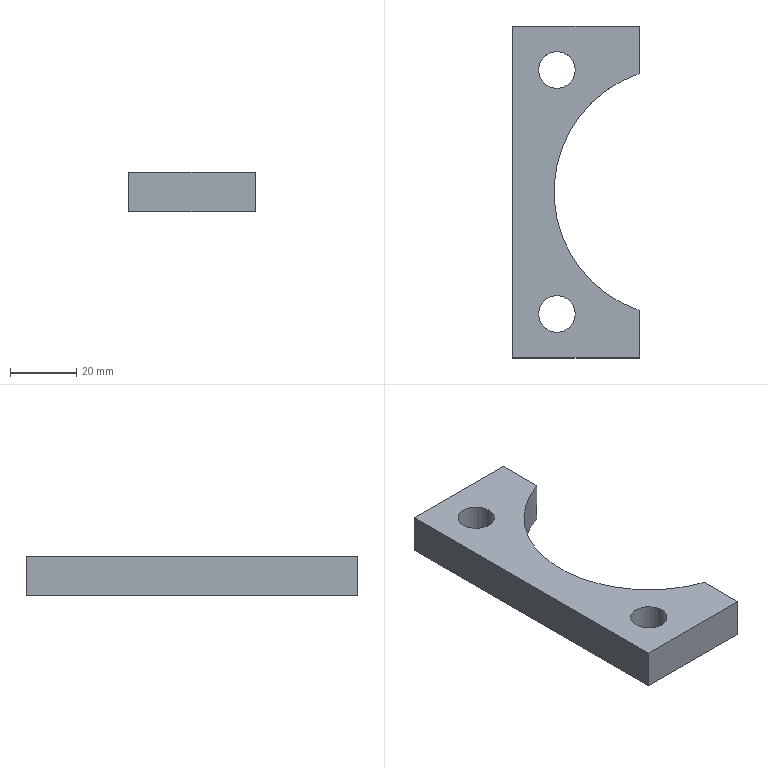Part | NX | features MAIN_BODY 2 | 1 solid | 10 faces | box 38 x 100 x 12 mm | volume 27313 mm3 | plane 7 | cylinder 3 | commonest cylinder face diameters 11 x2 75.2 x1
STEP:
#1=CARTESIAN_POINT('',(-682.,-155.634,390.));
#2=VERTEX_POINT('',#1);
#3=CARTESIAN_POINT('',(-682.,-170.,390.));
#4=VERTEX_POINT('',#3);
#5=CARTESIAN_POINT('',(-682.,-70.,390.));
#6=DIRECTION('',(0.,-1.,0.));
#7=VECTOR('',#6,1000.);
#8=LINE('',#5,#7);
#9=EDGE_CURVE('',#2,#4,#8,.T.);
#10=ORIENTED_EDGE('',*,*,#9,.T.);
#11=CARTESIAN_POINT('',(-682.,-170.,378.));
#12=VERTEX_POINT('',#11);
#13=CARTESIAN_POINT('',(-682.,-170.,378.));
#14=DIRECTION('',(0.,0.,1.));
#15=VECTOR('',#14,1000.);
#16=LINE('',#13,#15);
#17=EDGE_CURVE('',#12,#4,#16,.T.);
#18=ORIENTED_EDGE('',*,*,#17,.F.);
#19=CARTESIAN_POINT('',(-682.,-155.634,378.));
#20=VERTEX_POINT('',#19);
#21=CARTESIAN_POINT('',(-682.,-70.,378.));
#22=DIRECTION('',(0.,-1.,0.));
#23=VECTOR('',#22,1000.);
#24=LINE('',#21,#23);
#25=EDGE_CURVE('',#20,#12,#24,.T.);
#26=ORIENTED_EDGE('',*,*,#25,.F.);
#27=CARTESIAN_POINT('',(-682.,-155.634,378.));
#28=DIRECTION('',(0.,0.,1.));
#29=VECTOR('',#28,1000.);
#30=LINE('',#27,#29);
#31=EDGE_CURVE('',#2,#20,#30,.F.);
#32=ORIENTED_EDGE('',*,*,#31,.F.);
#33=EDGE_LOOP('',(#10,#18,#26,#32));
#34=FACE_BOUND('',#33,.T.);
#35=CARTESIAN_POINT('',(-682.,-70.,378.));
#36=DIRECTION('',(1.,0.,0.));
#37=DIRECTION('',(0.,1.,0.));
#38=AXIS2_PLACEMENT_3D('',#35,#36,#37);
#39=PLANE('',#38);
#40=ADVANCED_FACE('',(#34),#39,.T.);
#41=CARTESIAN_POINT('',(-682.,-70.,378.));
#42=VERTEX_POINT('',#41);
#43=CARTESIAN_POINT('',(-682.,-84.366,378.));
#44=VERTEX_POINT('',#43);
#45=CARTESIAN_POINT('',(-682.,-70.,378.));
#46=DIRECTION('',(0.,-1.,0.));
#47=VECTOR('',#46,1000.);
#48=LINE('',#45,#47);
#49=EDGE_CURVE('',#42,#44,#48,.T.);
#50=ORIENTED_EDGE('',*,*,#49,.F.);
#51=CARTESIAN_POINT('',(-682.,-70.,390.));
#52=VERTEX_POINT('',#51);
#53=CARTESIAN_POINT('',(-682.,-70.,378.));
#54=DIRECTION('',(0.,0.,1.));
#55=VECTOR('',#54,1000.);
#56=LINE('',#53,#55);
#57=EDGE_CURVE('',#42,#52,#56,.T.);
#58=ORIENTED_EDGE('',*,*,#57,.T.);
#59=CARTESIAN_POINT('',(-682.,-84.366,390.));
#60=VERTEX_POINT('',#59);
#61=CARTESIAN_POINT('',(-682.,-70.,390.));
#62=DIRECTION('',(0.,-1.,0.));
#63=VECTOR('',#62,1000.);
#64=LINE('',#61,#63);
#65=EDGE_CURVE('',#52,#60,#64,.T.);
#66=ORIENTED_EDGE('',*,*,#65,.T.);
#67=CARTESIAN_POINT('',(-682.,-84.366,378.));
#68=DIRECTION('',(0.,0.,1.));
#69=VECTOR('',#68,1000.);
#70=LINE('',#67,#69);
#71=EDGE_CURVE('',#44,#60,#70,.T.);
#72=ORIENTED_EDGE('',*,*,#71,.F.);
#73=EDGE_LOOP('',(#50,#58,#66,#72));
#74=FACE_BOUND('',#73,.T.);
#75=CARTESIAN_POINT('',(-682.,-70.,378.));
#76=DIRECTION('',(1.,0.,0.));
#77=DIRECTION('',(0.,1.,0.));
#78=AXIS2_PLACEMENT_3D('',#75,#76,#77);
#79=PLANE('',#78);
#80=ADVANCED_FACE('',(#74),#79,.T.);
#81=CARTESIAN_POINT('',(-701.25,-83.25,378.));
#82=VERTEX_POINT('',#81);
#83=CARTESIAN_POINT('',(-706.75,-83.25,378.));
#84=DIRECTION('',(0.,0.,1.));
#85=DIRECTION('',(1.,0.,0.));
#86=AXIS2_PLACEMENT_3D('',#83,#84,#85);
#87=CIRCLE('',#86,5.5);
#88=EDGE_CURVE('',#82,#82,#87,.T.);
#89=ORIENTED_EDGE('',*,*,#88,.T.);
#90=EDGE_LOOP('',(#89));
#91=FACE_BOUND('',#90,.T.);
#92=CARTESIAN_POINT('',(-701.25,-156.75,378.));
#93=VERTEX_POINT('',#92);
#94=CARTESIAN_POINT('',(-706.75,-156.75,378.));
#95=DIRECTION('',(0.,0.,-1.));
#96=DIRECTION('',(1.,0.,0.));
#97=AXIS2_PLACEMENT_3D('',#94,#95,#96);
#98=CIRCLE('',#97,5.5);
#99=EDGE_CURVE('',#93,#93,#98,.T.);
#100=ORIENTED_EDGE('',*,*,#99,.F.);
#101=EDGE_LOOP('',(#100));
#102=FACE_BOUND('',#101,.T.);
#103=CARTESIAN_POINT('',(-670.,-120.,378.));
#104=DIRECTION('',(0.,0.,1.));
#105=DIRECTION('',(1.,0.,0.));
#106=AXIS2_PLACEMENT_3D('',#103,#104,#105);
#107=CIRCLE('',#106,37.6);
#108=EDGE_CURVE('',#44,#20,#107,.T.);
#109=ORIENTED_EDGE('',*,*,#108,.T.);
#110=ORIENTED_EDGE('',*,*,#25,.T.);
#111=CARTESIAN_POINT('',(-720.,-170.,378.));
#112=VERTEX_POINT('',#111);
#113=CARTESIAN_POINT('',(-682.,-170.,378.));
#114=DIRECTION('',(-1.,0.,0.));
#115=VECTOR('',#114,1000.);
#116=LINE('',#113,#115);
#117=EDGE_CURVE('',#12,#112,#116,.T.);
#118=ORIENTED_EDGE('',*,*,#117,.T.);
#119=CARTESIAN_POINT('',(-720.,-70.,378.));
#120=VERTEX_POINT('',#119);
#121=CARTESIAN_POINT('',(-720.,-170.,378.));
#122=DIRECTION('',(0.,1.,0.));
#123=VECTOR('',#122,1000.);
#124=LINE('',#121,#123);
#125=EDGE_CURVE('',#112,#120,#124,.T.);
#126=ORIENTED_EDGE('',*,*,#125,.T.);
#127=CARTESIAN_POINT('',(-720.,-70.,378.));
#128=DIRECTION('',(1.,0.,0.));
#129=VECTOR('',#128,1000.);
#130=LINE('',#127,#129);
#131=EDGE_CURVE('',#120,#42,#130,.T.);
#132=ORIENTED_EDGE('',*,*,#131,.T.);
#133=ORIENTED_EDGE('',*,*,#49,.T.);
#134=EDGE_LOOP('',(#109,#110,#118,#126,#132,#133));
#135=FACE_BOUND('',#134,.T.);
#136=CARTESIAN_POINT('',(-682.,-170.,378.));
#137=DIRECTION('',(0.,0.,1.));
#138=DIRECTION('',(-1.,0.,0.));
#139=AXIS2_PLACEMENT_3D('',#136,#137,#138);
#140=PLANE('',#139);
#141=ADVANCED_FACE('',(#91,#102,#135),#140,.F.);
#142=CARTESIAN_POINT('',(-701.25,-83.25,390.));
#143=VERTEX_POINT('',#142);
#144=CARTESIAN_POINT('',(-706.75,-83.25,390.));
#145=DIRECTION('',(0.,0.,1.));
#146=DIRECTION('',(1.,0.,0.));
#147=AXIS2_PLACEMENT_3D('',#144,#145,#146);
#148=CIRCLE('',#147,5.5);
#149=EDGE_CURVE('',#143,#143,#148,.T.);
#150=ORIENTED_EDGE('',*,*,#149,.F.);
#151=EDGE_LOOP('',(#150));
#152=FACE_BOUND('',#151,.T.);
#153=CARTESIAN_POINT('',(-701.25,-156.75,390.));
#154=VERTEX_POINT('',#153);
#155=CARTESIAN_POINT('',(-706.75,-156.75,390.));
#156=DIRECTION('',(0.,0.,-1.));
#157=DIRECTION('',(1.,0.,0.));
#158=AXIS2_PLACEMENT_3D('',#155,#156,#157);
#159=CIRCLE('',#158,5.5);
#160=EDGE_CURVE('',#154,#154,#159,.T.);
#161=ORIENTED_EDGE('',*,*,#160,.T.);
#162=EDGE_LOOP('',(#161));
#163=FACE_BOUND('',#162,.T.);
#164=ORIENTED_EDGE('',*,*,#65,.F.);
#165=CARTESIAN_POINT('',(-720.,-70.,390.));
#166=VERTEX_POINT('',#165);
#167=CARTESIAN_POINT('',(-720.,-70.,390.));
#168=DIRECTION('',(1.,0.,0.));
#169=VECTOR('',#168,1000.);
#170=LINE('',#167,#169);
#171=EDGE_CURVE('',#166,#52,#170,.T.);
#172=ORIENTED_EDGE('',*,*,#171,.F.);
#173=CARTESIAN_POINT('',(-720.,-170.,390.));
#174=VERTEX_POINT('',#173);
#175=CARTESIAN_POINT('',(-720.,-170.,390.));
#176=DIRECTION('',(0.,1.,0.));
#177=VECTOR('',#176,1000.);
#178=LINE('',#175,#177);
#179=EDGE_CURVE('',#174,#166,#178,.T.);
#180=ORIENTED_EDGE('',*,*,#179,.F.);
#181=CARTESIAN_POINT('',(-682.,-170.,390.));
#182=DIRECTION('',(-1.,0.,0.));
#183=VECTOR('',#182,1000.);
#184=LINE('',#181,#183);
#185=EDGE_CURVE('',#4,#174,#184,.T.);
#186=ORIENTED_EDGE('',*,*,#185,.F.);
#187=ORIENTED_EDGE('',*,*,#9,.F.);
#188=CARTESIAN_POINT('',(-670.,-120.,390.));
#189=DIRECTION('',(0.,0.,1.));
#190=DIRECTION('',(1.,0.,0.));
#191=AXIS2_PLACEMENT_3D('',#188,#189,#190);
#192=CIRCLE('',#191,37.6);
#193=EDGE_CURVE('',#60,#2,#192,.T.);
#194=ORIENTED_EDGE('',*,*,#193,.F.);
#195=EDGE_LOOP('',(#164,#172,#180,#186,#187,#194));
#196=FACE_BOUND('',#195,.T.);
#197=CARTESIAN_POINT('',(-682.,-170.,390.));
#198=DIRECTION('',(0.,0.,1.));
#199=DIRECTION('',(-1.,0.,0.));
#200=AXIS2_PLACEMENT_3D('',#197,#198,#199);
#201=PLANE('',#200);
#202=ADVANCED_FACE('',(#152,#163,#196),#201,.T.);
#203=ORIENTED_EDGE('',*,*,#185,.T.);
#204=CARTESIAN_POINT('',(-720.,-170.,378.));
#205=DIRECTION('',(0.,0.,1.));
#206=VECTOR('',#205,1000.);
#207=LINE('',#204,#206);
#208=EDGE_CURVE('',#112,#174,#207,.T.);
#209=ORIENTED_EDGE('',*,*,#208,.F.);
#210=ORIENTED_EDGE('',*,*,#117,.F.);
#211=ORIENTED_EDGE('',*,*,#17,.T.);
#212=EDGE_LOOP('',(#203,#209,#210,#211));
#213=FACE_BOUND('',#212,.T.);
#214=CARTESIAN_POINT('',(-682.,-170.,378.));
#215=DIRECTION('',(0.,-1.,0.));
#216=DIRECTION('',(1.,0.,0.));
#217=AXIS2_PLACEMENT_3D('',#214,#215,#216);
#218=PLANE('',#217);
#219=ADVANCED_FACE('',(#213),#218,.T.);
#220=ORIENTED_EDGE('',*,*,#179,.T.);
#221=CARTESIAN_POINT('',(-720.,-70.,378.));
#222=DIRECTION('',(0.,0.,1.));
#223=VECTOR('',#222,1000.);
#224=LINE('',#221,#223);
#225=EDGE_CURVE('',#120,#166,#224,.T.);
#226=ORIENTED_EDGE('',*,*,#225,.F.);
#227=ORIENTED_EDGE('',*,*,#125,.F.);
#228=ORIENTED_EDGE('',*,*,#208,.T.);
#229=EDGE_LOOP('',(#220,#226,#227,#228));
#230=FACE_BOUND('',#229,.T.);
#231=CARTESIAN_POINT('',(-720.,-170.,378.));
#232=DIRECTION('',(-1.,0.,0.));
#233=DIRECTION('',(0.,-1.,0.));
#234=AXIS2_PLACEMENT_3D('',#231,#232,#233);
#235=PLANE('',#234);
#236=ADVANCED_FACE('',(#230),#235,.T.);
#237=ORIENTED_EDGE('',*,*,#99,.T.);
#238=EDGE_LOOP('',(#237));
#239=FACE_BOUND('',#238,.T.);
#240=ORIENTED_EDGE('',*,*,#160,.F.);
#241=EDGE_LOOP('',(#240));
#242=FACE_BOUND('',#241,.T.);
#243=CARTESIAN_POINT('',(-706.75,-156.75,378.));
#244=DIRECTION('',(0.,0.,1.));
#245=DIRECTION('',(-1.,0.,0.));
#246=AXIS2_PLACEMENT_3D('',#243,#244,#245);
#247=CYLINDRICAL_SURFACE('',#246,5.5);
#248=ADVANCED_FACE('',(#239,#242),#247,.F.);
#249=ORIENTED_EDGE('',*,*,#171,.T.);
#250=ORIENTED_EDGE('',*,*,#57,.F.);
#251=ORIENTED_EDGE('',*,*,#131,.F.);
#252=ORIENTED_EDGE('',*,*,#225,.T.);
#253=EDGE_LOOP('',(#249,#250,#251,#252));
#254=FACE_BOUND('',#253,.T.);
#255=CARTESIAN_POINT('',(-720.,-70.,378.));
#256=DIRECTION('',(0.,1.,0.));
#257=DIRECTION('',(0.,0.,-1.));
#258=AXIS2_PLACEMENT_3D('',#255,#256,#257);
#259=PLANE('',#258);
#260=ADVANCED_FACE('',(#254),#259,.T.);
#261=ORIENTED_EDGE('',*,*,#88,.F.);
#262=EDGE_LOOP('',(#261));
#263=FACE_BOUND('',#262,.T.);
#264=ORIENTED_EDGE('',*,*,#149,.T.);
#265=EDGE_LOOP('',(#264));
#266=FACE_BOUND('',#265,.T.);
#267=CARTESIAN_POINT('',(-706.75,-83.25,378.));
#268=DIRECTION('',(0.,0.,1.));
#269=DIRECTION('',(-1.,0.,0.));
#270=AXIS2_PLACEMENT_3D('',#267,#268,#269);
#271=CYLINDRICAL_SURFACE('',#270,5.5);
#272=ADVANCED_FACE('',(#263,#266),#271,.F.);
#273=ORIENTED_EDGE('',*,*,#193,.T.);
#274=ORIENTED_EDGE('',*,*,#31,.T.);
#275=ORIENTED_EDGE('',*,*,#108,.F.);
#276=ORIENTED_EDGE('',*,*,#71,.T.);
#277=EDGE_LOOP('',(#273,#274,#275,#276));
#278=FACE_BOUND('',#277,.T.);
#279=CARTESIAN_POINT('',(-670.,-120.,378.));
#280=DIRECTION('',(0.,0.,1.));
#281=DIRECTION('',(-1.,0.,0.));
#282=AXIS2_PLACEMENT_3D('',#279,#280,#281);
#283=CYLINDRICAL_SURFACE('',#282,37.6);
#284=ADVANCED_FACE('',(#278),#283,.F.);
#285=CLOSED_SHELL('',(#40,#80,#141,#202,#219,#236,#248,#260,#272,#284));
#286=MANIFOLD_SOLID_BREP('',#285);
#287=(LENGTH_UNIT()NAMED_UNIT(*)SI_UNIT(.MILLI.,.METRE.));
#288=UNCERTAINTY_MEASURE_WITH_UNIT(LENGTH_MEASURE(0.00001),#287,'','');
#289=(NAMED_UNIT(*)PLANE_ANGLE_UNIT()SI_UNIT($,.RADIAN.));
#290=(NAMED_UNIT(*)SI_UNIT($,.STERADIAN.)SOLID_ANGLE_UNIT());
#291=(GEOMETRIC_REPRESENTATION_CONTEXT(3)GLOBAL_UNCERTAINTY_ASSIGNED_CONTEXT((#288))GLOBAL_UNIT_ASSIGNED_CONTEXT((#287,#289,#290))REPRESENTATION_CONTEXT('',''));
#292=ADVANCED_BREP_SHAPE_REPRESENTATION('',(#286),#291);